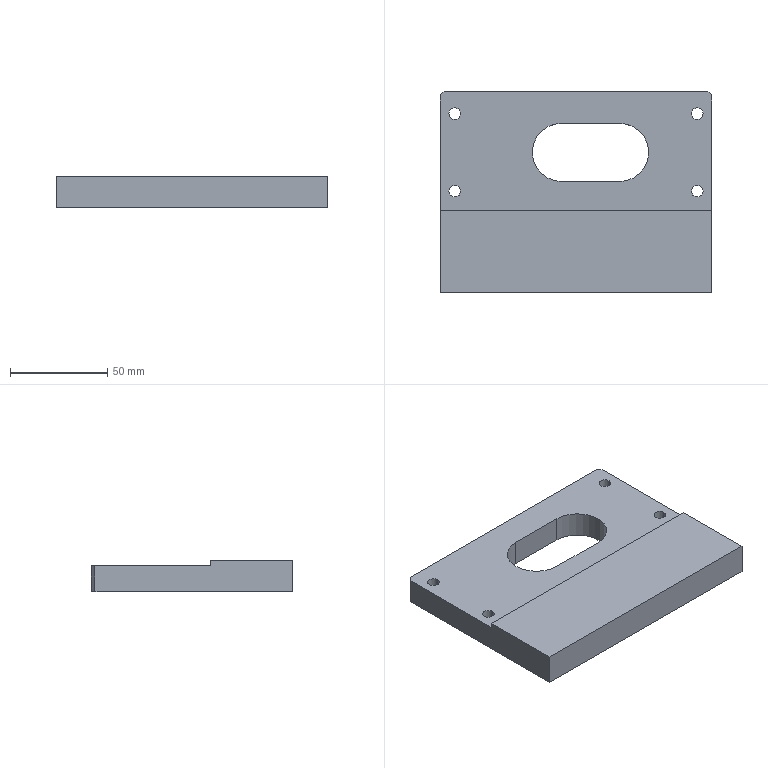Part | STEP file | [01]-2 | 1 solid | 22 faces | box 140 x 104 x 16 mm | volume 187092 mm3 | plane 12 | cylinder 10 | commonest cylinder face diameters 6 x8 30 x2
STEP:
#1=CARTESIAN_POINT('',(135.5,92.4,13.35));
#2=VERTEX_POINT('',#1);
#3=CARTESIAN_POINT('',(129.5,92.4,13.35));
#4=VERTEX_POINT('',#3);
#5=CARTESIAN_POINT('',(132.5,92.4,13.35));
#6=DIRECTION('',(0.,0.,-1.));
#7=DIRECTION('',(-1.,0.,0.));
#8=AXIS2_PLACEMENT_3D('',#5,#6,#7);
#9=CIRCLE('',#8,3.);
#10=EDGE_CURVE('',#2,#4,#9,.T.);
#11=ORIENTED_EDGE('',*,*,#10,.F.);
#12=CARTESIAN_POINT('',(135.5,92.4,0.));
#13=VERTEX_POINT('',#12);
#14=CARTESIAN_POINT('',(135.5,92.4,13.35));
#15=DIRECTION('',(0.,0.,-1.));
#16=VECTOR('',#15,1000.);
#17=LINE('',#14,#16);
#18=EDGE_CURVE('',#2,#13,#17,.T.);
#19=ORIENTED_EDGE('',*,*,#18,.T.);
#20=CARTESIAN_POINT('',(129.5,92.4,0.));
#21=VERTEX_POINT('',#20);
#22=CARTESIAN_POINT('',(132.5,92.4,0.));
#23=DIRECTION('',(0.,0.,1.));
#24=DIRECTION('',(1.,0.,0.));
#25=AXIS2_PLACEMENT_3D('',#22,#23,#24);
#26=CIRCLE('',#25,3.);
#27=EDGE_CURVE('',#21,#13,#26,.T.);
#28=ORIENTED_EDGE('',*,*,#27,.F.);
#29=CARTESIAN_POINT('',(129.5,92.4,13.35));
#30=DIRECTION('',(0.,0.,-1.));
#31=VECTOR('',#30,1000.);
#32=LINE('',#29,#31);
#33=EDGE_CURVE('',#4,#21,#32,.T.);
#34=ORIENTED_EDGE('',*,*,#33,.F.);
#35=EDGE_LOOP('',(#11,#19,#28,#34));
#36=FACE_OUTER_BOUND('',#35,.T.);
#37=CARTESIAN_POINT('',(132.5,92.4,13.35));
#38=DIRECTION('',(0.,0.,-1.));
#39=DIRECTION('',(-1.,0.,0.));
#40=AXIS2_PLACEMENT_3D('',#37,#38,#39);
#41=CYLINDRICAL_SURFACE('',#40,3.);
#42=ADVANCED_FACE('',(#36),#41,.F.);
#43=CARTESIAN_POINT('',(135.5,52.4,13.35));
#44=VERTEX_POINT('',#43);
#45=CARTESIAN_POINT('',(129.5,52.4,13.35));
#46=VERTEX_POINT('',#45);
#47=CARTESIAN_POINT('',(132.5,52.4,13.35));
#48=DIRECTION('',(0.,0.,-1.));
#49=DIRECTION('',(-1.,0.,0.));
#50=AXIS2_PLACEMENT_3D('',#47,#48,#49);
#51=CIRCLE('',#50,3.);
#52=EDGE_CURVE('',#44,#46,#51,.T.);
#53=ORIENTED_EDGE('',*,*,#52,.F.);
#54=CARTESIAN_POINT('',(135.5,52.4,0.));
#55=VERTEX_POINT('',#54);
#56=CARTESIAN_POINT('',(135.5,52.4,13.35));
#57=DIRECTION('',(0.,0.,-1.));
#58=VECTOR('',#57,1000.);
#59=LINE('',#56,#58);
#60=EDGE_CURVE('',#44,#55,#59,.T.);
#61=ORIENTED_EDGE('',*,*,#60,.T.);
#62=CARTESIAN_POINT('',(129.5,52.4,0.));
#63=VERTEX_POINT('',#62);
#64=CARTESIAN_POINT('',(132.5,52.4,0.));
#65=DIRECTION('',(0.,0.,1.));
#66=DIRECTION('',(1.,0.,0.));
#67=AXIS2_PLACEMENT_3D('',#64,#65,#66);
#68=CIRCLE('',#67,3.);
#69=EDGE_CURVE('',#63,#55,#68,.T.);
#70=ORIENTED_EDGE('',*,*,#69,.F.);
#71=CARTESIAN_POINT('',(129.5,52.4,13.35));
#72=DIRECTION('',(0.,0.,-1.));
#73=VECTOR('',#72,1000.);
#74=LINE('',#71,#73);
#75=EDGE_CURVE('',#46,#63,#74,.T.);
#76=ORIENTED_EDGE('',*,*,#75,.F.);
#77=EDGE_LOOP('',(#53,#61,#70,#76));
#78=FACE_OUTER_BOUND('',#77,.T.);
#79=CARTESIAN_POINT('',(132.5,52.4,13.35));
#80=DIRECTION('',(0.,0.,-1.));
#81=DIRECTION('',(-1.,0.,0.));
#82=AXIS2_PLACEMENT_3D('',#79,#80,#81);
#83=CYLINDRICAL_SURFACE('',#82,3.);
#84=ADVANCED_FACE('',(#78),#83,.F.);
#85=CARTESIAN_POINT('',(10.5,52.4,13.35));
#86=VERTEX_POINT('',#85);
#87=CARTESIAN_POINT('',(4.5,52.4,13.35));
#88=VERTEX_POINT('',#87);
#89=CARTESIAN_POINT('',(7.5,52.4,13.35));
#90=DIRECTION('',(0.,0.,-1.));
#91=DIRECTION('',(-1.,0.,0.));
#92=AXIS2_PLACEMENT_3D('',#89,#90,#91);
#93=CIRCLE('',#92,3.);
#94=EDGE_CURVE('',#86,#88,#93,.T.);
#95=ORIENTED_EDGE('',*,*,#94,.F.);
#96=CARTESIAN_POINT('',(10.5,52.4,0.));
#97=VERTEX_POINT('',#96);
#98=CARTESIAN_POINT('',(10.5,52.4,13.35));
#99=DIRECTION('',(0.,0.,-1.));
#100=VECTOR('',#99,1000.);
#101=LINE('',#98,#100);
#102=EDGE_CURVE('',#86,#97,#101,.T.);
#103=ORIENTED_EDGE('',*,*,#102,.T.);
#104=CARTESIAN_POINT('',(4.5,52.4,0.));
#105=VERTEX_POINT('',#104);
#106=CARTESIAN_POINT('',(7.5,52.4,0.));
#107=DIRECTION('',(0.,0.,1.));
#108=DIRECTION('',(1.,0.,0.));
#109=AXIS2_PLACEMENT_3D('',#106,#107,#108);
#110=CIRCLE('',#109,3.);
#111=EDGE_CURVE('',#105,#97,#110,.T.);
#112=ORIENTED_EDGE('',*,*,#111,.F.);
#113=CARTESIAN_POINT('',(4.5,52.4,13.35));
#114=DIRECTION('',(0.,0.,-1.));
#115=VECTOR('',#114,1000.);
#116=LINE('',#113,#115);
#117=EDGE_CURVE('',#88,#105,#116,.T.);
#118=ORIENTED_EDGE('',*,*,#117,.F.);
#119=EDGE_LOOP('',(#95,#103,#112,#118));
#120=FACE_OUTER_BOUND('',#119,.T.);
#121=CARTESIAN_POINT('',(7.5,52.4,13.35));
#122=DIRECTION('',(0.,0.,-1.));
#123=DIRECTION('',(-1.,0.,0.));
#124=AXIS2_PLACEMENT_3D('',#121,#122,#123);
#125=CYLINDRICAL_SURFACE('',#124,3.);
#126=ADVANCED_FACE('',(#120),#125,.F.);
#127=CARTESIAN_POINT('',(10.5,92.4,13.35));
#128=VERTEX_POINT('',#127);
#129=CARTESIAN_POINT('',(4.5,92.4,13.35));
#130=VERTEX_POINT('',#129);
#131=CARTESIAN_POINT('',(7.5,92.4,13.35));
#132=DIRECTION('',(0.,0.,-1.));
#133=DIRECTION('',(-1.,0.,0.));
#134=AXIS2_PLACEMENT_3D('',#131,#132,#133);
#135=CIRCLE('',#134,3.);
#136=EDGE_CURVE('',#128,#130,#135,.T.);
#137=ORIENTED_EDGE('',*,*,#136,.F.);
#138=CARTESIAN_POINT('',(10.5,92.4,0.));
#139=VERTEX_POINT('',#138);
#140=CARTESIAN_POINT('',(10.5,92.4,13.35));
#141=DIRECTION('',(0.,0.,-1.));
#142=VECTOR('',#141,1000.);
#143=LINE('',#140,#142);
#144=EDGE_CURVE('',#128,#139,#143,.T.);
#145=ORIENTED_EDGE('',*,*,#144,.T.);
#146=CARTESIAN_POINT('',(4.5,92.4,0.));
#147=VERTEX_POINT('',#146);
#148=CARTESIAN_POINT('',(7.5,92.4,0.));
#149=DIRECTION('',(0.,0.,1.));
#150=DIRECTION('',(1.,0.,0.));
#151=AXIS2_PLACEMENT_3D('',#148,#149,#150);
#152=CIRCLE('',#151,3.);
#153=EDGE_CURVE('',#147,#139,#152,.T.);
#154=ORIENTED_EDGE('',*,*,#153,.F.);
#155=CARTESIAN_POINT('',(4.5,92.4,13.35));
#156=DIRECTION('',(0.,0.,-1.));
#157=VECTOR('',#156,1000.);
#158=LINE('',#155,#157);
#159=EDGE_CURVE('',#130,#147,#158,.T.);
#160=ORIENTED_EDGE('',*,*,#159,.F.);
#161=EDGE_LOOP('',(#137,#145,#154,#160));
#162=FACE_OUTER_BOUND('',#161,.T.);
#163=CARTESIAN_POINT('',(7.5,92.4,13.35));
#164=DIRECTION('',(0.,0.,-1.));
#165=DIRECTION('',(-1.,0.,0.));
#166=AXIS2_PLACEMENT_3D('',#163,#164,#165);
#167=CYLINDRICAL_SURFACE('',#166,3.);
#168=ADVANCED_FACE('',(#162),#167,.F.);
#169=CARTESIAN_POINT('',(138.,104.,13.35));
#170=VERTEX_POINT('',#169);
#171=CARTESIAN_POINT('',(2.,104.,13.35));
#172=VERTEX_POINT('',#171);
#173=CARTESIAN_POINT('',(0.,104.,13.35));
#174=DIRECTION('',(-1.,0.,0.));
#175=VECTOR('',#174,1000.);
#176=LINE('',#173,#175);
#177=EDGE_CURVE('',#170,#172,#176,.T.);
#178=ORIENTED_EDGE('',*,*,#177,.F.);
#179=CARTESIAN_POINT('',(138.,104.,0.));
#180=VERTEX_POINT('',#179);
#181=CARTESIAN_POINT('',(138.,104.,0.));
#182=DIRECTION('',(0.,0.,-1.));
#183=VECTOR('',#182,1000.);
#184=LINE('',#181,#183);
#185=EDGE_CURVE('',#170,#180,#184,.T.);
#186=ORIENTED_EDGE('',*,*,#185,.T.);
#187=CARTESIAN_POINT('',(2.,104.,0.));
#188=VERTEX_POINT('',#187);
#189=CARTESIAN_POINT('',(0.,104.,0.));
#190=DIRECTION('',(1.,0.,0.));
#191=VECTOR('',#190,1000.);
#192=LINE('',#189,#191);
#193=EDGE_CURVE('',#188,#180,#192,.T.);
#194=ORIENTED_EDGE('',*,*,#193,.F.);
#195=CARTESIAN_POINT('',(2.,104.,16.));
#196=DIRECTION('',(0.,0.,1.));
#197=VECTOR('',#196,1000.);
#198=LINE('',#195,#197);
#199=EDGE_CURVE('',#188,#172,#198,.T.);
#200=ORIENTED_EDGE('',*,*,#199,.T.);
#201=EDGE_LOOP('',(#178,#186,#194,#200));
#202=FACE_OUTER_BOUND('',#201,.T.);
#203=CARTESIAN_POINT('',(0.,104.,0.));
#204=DIRECTION('',(0.,1.,0.));
#205=DIRECTION('',(-1.,0.,0.));
#206=AXIS2_PLACEMENT_3D('',#203,#204,#205);
#207=PLANE('',#206);
#208=ADVANCED_FACE('',(#202),#207,.T.);
#209=CARTESIAN_POINT('',(0.,42.4,16.));
#210=VERTEX_POINT('',#209);
#211=CARTESIAN_POINT('',(140.,42.4,16.));
#212=VERTEX_POINT('',#211);
#213=CARTESIAN_POINT('',(0.,42.4,16.));
#214=DIRECTION('',(1.,0.,0.));
#215=VECTOR('',#214,1000.);
#216=LINE('',#213,#215);
#217=EDGE_CURVE('',#210,#212,#216,.T.);
#218=ORIENTED_EDGE('',*,*,#217,.F.);
#219=CARTESIAN_POINT('',(0.,0.,16.));
#220=VERTEX_POINT('',#219);
#221=CARTESIAN_POINT('',(0.,104.,16.));
#222=DIRECTION('',(0.,-1.,0.));
#223=VECTOR('',#222,1000.);
#224=LINE('',#221,#223);
#225=EDGE_CURVE('',#210,#220,#224,.T.);
#226=ORIENTED_EDGE('',*,*,#225,.T.);
#227=CARTESIAN_POINT('',(140.,0.,16.));
#228=VERTEX_POINT('',#227);
#229=CARTESIAN_POINT('',(0.,0.,16.));
#230=DIRECTION('',(1.,0.,0.));
#231=VECTOR('',#230,1000.);
#232=LINE('',#229,#231);
#233=EDGE_CURVE('',#220,#228,#232,.T.);
#234=ORIENTED_EDGE('',*,*,#233,.T.);
#235=CARTESIAN_POINT('',(140.,104.,16.));
#236=DIRECTION('',(0.,-1.,0.));
#237=VECTOR('',#236,1000.);
#238=LINE('',#235,#237);
#239=EDGE_CURVE('',#212,#228,#238,.T.);
#240=ORIENTED_EDGE('',*,*,#239,.F.);
#241=EDGE_LOOP('',(#218,#226,#234,#240));
#242=FACE_OUTER_BOUND('',#241,.T.);
#243=CARTESIAN_POINT('',(0.,104.,16.));
#244=DIRECTION('',(0.,0.,1.));
#245=DIRECTION('',(0.,-1.,0.));
#246=AXIS2_PLACEMENT_3D('',#243,#244,#245);
#247=PLANE('',#246);
#248=ADVANCED_FACE('',(#242),#247,.T.);
#249=CARTESIAN_POINT('',(140.,0.,0.));
#250=VERTEX_POINT('',#249);
#251=CARTESIAN_POINT('',(140.,0.,16.));
#252=DIRECTION('',(0.,0.,-1.));
#253=VECTOR('',#252,1000.);
#254=LINE('',#251,#253);
#255=EDGE_CURVE('',#228,#250,#254,.T.);
#256=ORIENTED_EDGE('',*,*,#255,.F.);
#257=ORIENTED_EDGE('',*,*,#233,.F.);
#258=CARTESIAN_POINT('',(0.,0.,0.));
#259=VERTEX_POINT('',#258);
#260=CARTESIAN_POINT('',(0.,0.,16.));
#261=DIRECTION('',(0.,0.,-1.));
#262=VECTOR('',#261,1000.);
#263=LINE('',#260,#262);
#264=EDGE_CURVE('',#220,#259,#263,.T.);
#265=ORIENTED_EDGE('',*,*,#264,.T.);
#266=CARTESIAN_POINT('',(0.,0.,0.));
#267=DIRECTION('',(1.,0.,0.));
#268=VECTOR('',#267,1000.);
#269=LINE('',#266,#268);
#270=EDGE_CURVE('',#259,#250,#269,.T.);
#271=ORIENTED_EDGE('',*,*,#270,.T.);
#272=EDGE_LOOP('',(#256,#257,#265,#271));
#273=FACE_OUTER_BOUND('',#272,.T.);
#274=CARTESIAN_POINT('',(0.,0.,16.));
#275=DIRECTION('',(0.,-1.,0.));
#276=DIRECTION('',(1.,0.,0.));
#277=AXIS2_PLACEMENT_3D('',#274,#275,#276);
#278=PLANE('',#277);
#279=ADVANCED_FACE('',(#273),#278,.T.);
#280=ORIENTED_EDGE('',*,*,#27,.T.);
#281=CARTESIAN_POINT('',(132.5,92.4,0.));
#282=DIRECTION('',(0.,0.,1.));
#283=DIRECTION('',(1.,0.,0.));
#284=AXIS2_PLACEMENT_3D('',#281,#282,#283);
#285=CIRCLE('',#284,3.);
#286=EDGE_CURVE('',#13,#21,#285,.T.);
#287=ORIENTED_EDGE('',*,*,#286,.T.);
#288=EDGE_LOOP('',(#280,#287));
#289=FACE_BOUND('',#288,.T.);
#290=ORIENTED_EDGE('',*,*,#69,.T.);
#291=CARTESIAN_POINT('',(132.5,52.4,0.));
#292=DIRECTION('',(0.,0.,1.));
#293=DIRECTION('',(1.,0.,0.));
#294=AXIS2_PLACEMENT_3D('',#291,#292,#293);
#295=CIRCLE('',#294,3.);
#296=EDGE_CURVE('',#55,#63,#295,.T.);
#297=ORIENTED_EDGE('',*,*,#296,.T.);
#298=EDGE_LOOP('',(#290,#297));
#299=FACE_BOUND('',#298,.T.);
#300=ORIENTED_EDGE('',*,*,#111,.T.);
#301=CARTESIAN_POINT('',(7.5,52.4,0.));
#302=DIRECTION('',(0.,0.,1.));
#303=DIRECTION('',(1.,0.,0.));
#304=AXIS2_PLACEMENT_3D('',#301,#302,#303);
#305=CIRCLE('',#304,3.);
#306=EDGE_CURVE('',#97,#105,#305,.T.);
#307=ORIENTED_EDGE('',*,*,#306,.T.);
#308=EDGE_LOOP('',(#300,#307));
#309=FACE_BOUND('',#308,.T.);
#310=ORIENTED_EDGE('',*,*,#153,.T.);
#311=CARTESIAN_POINT('',(7.5,92.4,0.));
#312=DIRECTION('',(0.,0.,1.));
#313=DIRECTION('',(1.,0.,0.));
#314=AXIS2_PLACEMENT_3D('',#311,#312,#313);
#315=CIRCLE('',#314,3.);
#316=EDGE_CURVE('',#139,#147,#315,.T.);
#317=ORIENTED_EDGE('',*,*,#316,.T.);
#318=EDGE_LOOP('',(#310,#317));
#319=FACE_BOUND('',#318,.T.);
#320=CARTESIAN_POINT('',(62.5,87.4,0.));
#321=VERTEX_POINT('',#320);
#322=CARTESIAN_POINT('',(62.5,57.4,0.));
#323=VERTEX_POINT('',#322);
#324=CARTESIAN_POINT('',(62.5,72.4,0.));
#325=DIRECTION('',(0.,0.,1.));
#326=DIRECTION('',(0.,1.,0.));
#327=AXIS2_PLACEMENT_3D('',#324,#325,#326);
#328=CIRCLE('',#327,15.);
#329=EDGE_CURVE('',#321,#323,#328,.T.);
#330=ORIENTED_EDGE('',*,*,#329,.T.);
#331=CARTESIAN_POINT('',(92.5,57.4,0.));
#332=VERTEX_POINT('',#331);
#333=CARTESIAN_POINT('',(0.,57.4,0.));
#334=DIRECTION('',(-1.,0.,0.));
#335=VECTOR('',#334,1000.);
#336=LINE('',#333,#335);
#337=EDGE_CURVE('',#332,#323,#336,.T.);
#338=ORIENTED_EDGE('',*,*,#337,.F.);
#339=CARTESIAN_POINT('',(92.5,87.4,0.));
#340=VERTEX_POINT('',#339);
#341=CARTESIAN_POINT('',(92.5,72.4,0.));
#342=DIRECTION('',(0.,0.,1.));
#343=DIRECTION('',(0.,1.,0.));
#344=AXIS2_PLACEMENT_3D('',#341,#342,#343);
#345=CIRCLE('',#344,15.);
#346=EDGE_CURVE('',#332,#340,#345,.T.);
#347=ORIENTED_EDGE('',*,*,#346,.T.);
#348=CARTESIAN_POINT('',(0.,87.4,0.));
#349=DIRECTION('',(1.,0.,0.));
#350=VECTOR('',#349,1000.);
#351=LINE('',#348,#350);
#352=EDGE_CURVE('',#321,#340,#351,.T.);
#353=ORIENTED_EDGE('',*,*,#352,.F.);
#354=EDGE_LOOP('',(#330,#338,#347,#353));
#355=FACE_BOUND('',#354,.T.);
#356=CARTESIAN_POINT('',(0.,102.,0.));
#357=VERTEX_POINT('',#356);
#358=CARTESIAN_POINT('',(0.,0.,0.));
#359=DIRECTION('',(0.,1.,0.));
#360=VECTOR('',#359,1000.);
#361=LINE('',#358,#360);
#362=EDGE_CURVE('',#259,#357,#361,.T.);
#363=ORIENTED_EDGE('',*,*,#362,.T.);
#364=CARTESIAN_POINT('',(-51.,51.,0.));
#365=DIRECTION('',(0.7071,0.7071,0.));
#366=VECTOR('',#365,1000.);
#367=LINE('',#364,#366);
#368=EDGE_CURVE('',#357,#188,#367,.T.);
#369=ORIENTED_EDGE('',*,*,#368,.T.);
#370=ORIENTED_EDGE('',*,*,#193,.T.);
#371=CARTESIAN_POINT('',(140.,102.,0.));
#372=VERTEX_POINT('',#371);
#373=CARTESIAN_POINT('',(121.,121.,0.));
#374=DIRECTION('',(0.7071,-0.7071,0.));
#375=VECTOR('',#374,1000.);
#376=LINE('',#373,#375);
#377=EDGE_CURVE('',#180,#372,#376,.T.);
#378=ORIENTED_EDGE('',*,*,#377,.T.);
#379=CARTESIAN_POINT('',(140.,0.,0.));
#380=DIRECTION('',(0.,1.,0.));
#381=VECTOR('',#380,1000.);
#382=LINE('',#379,#381);
#383=EDGE_CURVE('',#250,#372,#382,.T.);
#384=ORIENTED_EDGE('',*,*,#383,.F.);
#385=ORIENTED_EDGE('',*,*,#270,.F.);
#386=EDGE_LOOP('',(#363,#369,#370,#378,#384,#385));
#387=FACE_OUTER_BOUND('',#386,.T.);
#388=CARTESIAN_POINT('',(0.,0.,0.));
#389=DIRECTION('',(0.,0.,-1.));
#390=DIRECTION('',(0.,1.,0.));
#391=AXIS2_PLACEMENT_3D('',#388,#389,#390);
#392=PLANE('',#391);
#393=ADVANCED_FACE('',(#289,#299,#309,#319,#355,#387),#392,.T.);
#394=ORIENTED_EDGE('',*,*,#225,.F.);
#395=CARTESIAN_POINT('',(0.,42.4,13.35));
#396=VERTEX_POINT('',#395);
#397=CARTESIAN_POINT('',(0.,42.4,-87.886));
#398=DIRECTION('',(0.,0.,-1.));
#399=VECTOR('',#398,1000.);
#400=LINE('',#397,#399);
#401=EDGE_CURVE('',#210,#396,#400,.T.);
#402=ORIENTED_EDGE('',*,*,#401,.T.);
#403=CARTESIAN_POINT('',(0.,102.,13.35));
#404=VERTEX_POINT('',#403);
#405=CARTESIAN_POINT('',(0.,329.827,13.35));
#406=DIRECTION('',(0.,1.,0.));
#407=VECTOR('',#406,1000.);
#408=LINE('',#405,#407);
#409=EDGE_CURVE('',#396,#404,#408,.T.);
#410=ORIENTED_EDGE('',*,*,#409,.T.);
#411=CARTESIAN_POINT('',(0.,102.,0.));
#412=DIRECTION('',(0.,0.,-1.));
#413=VECTOR('',#412,1000.);
#414=LINE('',#411,#413);
#415=EDGE_CURVE('',#404,#357,#414,.T.);
#416=ORIENTED_EDGE('',*,*,#415,.T.);
#417=ORIENTED_EDGE('',*,*,#362,.F.);
#418=ORIENTED_EDGE('',*,*,#264,.F.);
#419=EDGE_LOOP('',(#394,#402,#410,#416,#417,#418));
#420=FACE_OUTER_BOUND('',#419,.T.);
#421=CARTESIAN_POINT('',(0.,329.827,-87.886));
#422=DIRECTION('',(1.,0.,0.));
#423=DIRECTION('',(0.,1.,0.));
#424=AXIS2_PLACEMENT_3D('',#421,#422,#423);
#425=PLANE('',#424);
#426=ADVANCED_FACE('',(#420),#425,.F.);
#427=CARTESIAN_POINT('',(140.,42.4,13.35));
#428=VERTEX_POINT('',#427);
#429=CARTESIAN_POINT('',(140.,102.,13.35));
#430=VERTEX_POINT('',#429);
#431=CARTESIAN_POINT('',(140.,81.4,13.35));
#432=DIRECTION('',(0.,1.,0.));
#433=VECTOR('',#432,1000.);
#434=LINE('',#431,#433);
#435=EDGE_CURVE('',#428,#430,#434,.T.);
#436=ORIENTED_EDGE('',*,*,#435,.F.);
#437=CARTESIAN_POINT('',(140.,42.4,13.35));
#438=DIRECTION('',(0.,0.,1.));
#439=VECTOR('',#438,1000.);
#440=LINE('',#437,#439);
#441=EDGE_CURVE('',#428,#212,#440,.T.);
#442=ORIENTED_EDGE('',*,*,#441,.T.);
#443=ORIENTED_EDGE('',*,*,#239,.T.);
#444=ORIENTED_EDGE('',*,*,#255,.T.);
#445=ORIENTED_EDGE('',*,*,#383,.T.);
#446=CARTESIAN_POINT('',(140.,102.,-87.886));
#447=DIRECTION('',(0.,0.,1.));
#448=VECTOR('',#447,1000.);
#449=LINE('',#446,#448);
#450=EDGE_CURVE('',#372,#430,#449,.T.);
#451=ORIENTED_EDGE('',*,*,#450,.T.);
#452=EDGE_LOOP('',(#436,#442,#443,#444,#445,#451));
#453=FACE_OUTER_BOUND('',#452,.T.);
#454=CARTESIAN_POINT('',(140.,329.827,-87.886));
#455=DIRECTION('',(1.,0.,0.));
#456=DIRECTION('',(0.,1.,0.));
#457=AXIS2_PLACEMENT_3D('',#454,#455,#456);
#458=PLANE('',#457);
#459=ADVANCED_FACE('',(#453),#458,.T.);
#460=CARTESIAN_POINT('',(140.,102.,13.35));
#461=DIRECTION('',(-0.7071,0.7071,0.));
#462=VECTOR('',#461,1000.);
#463=LINE('',#460,#462);
#464=EDGE_CURVE('',#430,#170,#463,.T.);
#465=ORIENTED_EDGE('',*,*,#464,.F.);
#466=ORIENTED_EDGE('',*,*,#450,.F.);
#467=ORIENTED_EDGE('',*,*,#377,.F.);
#468=ORIENTED_EDGE('',*,*,#185,.F.);
#469=EDGE_LOOP('',(#465,#466,#467,#468));
#470=FACE_OUTER_BOUND('',#469,.T.);
#471=CARTESIAN_POINT('',(140.,102.,-87.886));
#472=DIRECTION('',(-0.7071,-0.7071,0.));
#473=DIRECTION('',(0.,0.,1.));
#474=AXIS2_PLACEMENT_3D('',#471,#472,#473);
#475=PLANE('',#474);
#476=ADVANCED_FACE('',(#470),#475,.F.);
#477=CARTESIAN_POINT('',(2.,104.,13.35));
#478=DIRECTION('',(-0.7071,-0.7071,0.));
#479=VECTOR('',#478,1000.);
#480=LINE('',#477,#479);
#481=EDGE_CURVE('',#172,#404,#480,.T.);
#482=ORIENTED_EDGE('',*,*,#481,.F.);
#483=ORIENTED_EDGE('',*,*,#199,.F.);
#484=ORIENTED_EDGE('',*,*,#368,.F.);
#485=ORIENTED_EDGE('',*,*,#415,.F.);
#486=EDGE_LOOP('',(#482,#483,#484,#485));
#487=FACE_OUTER_BOUND('',#486,.T.);
#488=CARTESIAN_POINT('',(2.,104.,0.));
#489=DIRECTION('',(-0.7071,0.7071,0.));
#490=DIRECTION('',(0.,0.,-1.));
#491=AXIS2_PLACEMENT_3D('',#488,#489,#490);
#492=PLANE('',#491);
#493=ADVANCED_FACE('',(#487),#492,.T.);
#494=CARTESIAN_POINT('',(132.5,92.4,13.35));
#495=DIRECTION('',(0.,0.,-1.));
#496=DIRECTION('',(-1.,0.,0.));
#497=AXIS2_PLACEMENT_3D('',#494,#495,#496);
#498=CIRCLE('',#497,3.);
#499=EDGE_CURVE('',#4,#2,#498,.T.);
#500=ORIENTED_EDGE('',*,*,#499,.T.);
#501=ORIENTED_EDGE('',*,*,#10,.T.);
#502=EDGE_LOOP('',(#500,#501));
#503=FACE_BOUND('',#502,.T.);
#504=CARTESIAN_POINT('',(132.5,52.4,13.35));
#505=DIRECTION('',(0.,0.,-1.));
#506=DIRECTION('',(-1.,0.,0.));
#507=AXIS2_PLACEMENT_3D('',#504,#505,#506);
#508=CIRCLE('',#507,3.);
#509=EDGE_CURVE('',#46,#44,#508,.T.);
#510=ORIENTED_EDGE('',*,*,#509,.T.);
#511=ORIENTED_EDGE('',*,*,#52,.T.);
#512=EDGE_LOOP('',(#510,#511));
#513=FACE_BOUND('',#512,.T.);
#514=CARTESIAN_POINT('',(7.5,52.4,13.35));
#515=DIRECTION('',(0.,0.,-1.));
#516=DIRECTION('',(-1.,0.,0.));
#517=AXIS2_PLACEMENT_3D('',#514,#515,#516);
#518=CIRCLE('',#517,3.);
#519=EDGE_CURVE('',#88,#86,#518,.T.);
#520=ORIENTED_EDGE('',*,*,#519,.T.);
#521=ORIENTED_EDGE('',*,*,#94,.T.);
#522=EDGE_LOOP('',(#520,#521));
#523=FACE_BOUND('',#522,.T.);
#524=CARTESIAN_POINT('',(7.5,92.4,13.35));
#525=DIRECTION('',(0.,0.,-1.));
#526=DIRECTION('',(-1.,0.,0.));
#527=AXIS2_PLACEMENT_3D('',#524,#525,#526);
#528=CIRCLE('',#527,3.);
#529=EDGE_CURVE('',#130,#128,#528,.T.);
#530=ORIENTED_EDGE('',*,*,#529,.T.);
#531=ORIENTED_EDGE('',*,*,#136,.T.);
#532=EDGE_LOOP('',(#530,#531));
#533=FACE_BOUND('',#532,.T.);
#534=ORIENTED_EDGE('',*,*,#464,.T.);
#535=ORIENTED_EDGE('',*,*,#177,.T.);
#536=ORIENTED_EDGE('',*,*,#481,.T.);
#537=ORIENTED_EDGE('',*,*,#409,.F.);
#538=CARTESIAN_POINT('',(55.,42.4,13.35));
#539=DIRECTION('',(1.,0.,0.));
#540=VECTOR('',#539,1000.);
#541=LINE('',#538,#540);
#542=EDGE_CURVE('',#396,#428,#541,.T.);
#543=ORIENTED_EDGE('',*,*,#542,.T.);
#544=ORIENTED_EDGE('',*,*,#435,.T.);
#545=EDGE_LOOP('',(#534,#535,#536,#537,#543,#544));
#546=FACE_OUTER_BOUND('',#545,.T.);
#547=CARTESIAN_POINT('',(92.5,57.4,13.35));
#548=VERTEX_POINT('',#547);
#549=CARTESIAN_POINT('',(62.5,57.4,13.35));
#550=VERTEX_POINT('',#549);
#551=CARTESIAN_POINT('',(77.5,57.4,13.35));
#552=DIRECTION('',(-1.,0.,0.));
#553=VECTOR('',#552,1000.);
#554=LINE('',#551,#553);
#555=EDGE_CURVE('',#548,#550,#554,.T.);
#556=ORIENTED_EDGE('',*,*,#555,.T.);
#557=CARTESIAN_POINT('',(62.5,87.4,13.35));
#558=VERTEX_POINT('',#557);
#559=CARTESIAN_POINT('',(62.5,72.4,13.35));
#560=DIRECTION('',(0.,0.,-1.));
#561=DIRECTION('',(0.,1.,0.));
#562=AXIS2_PLACEMENT_3D('',#559,#560,#561);
#563=CIRCLE('',#562,15.);
#564=EDGE_CURVE('',#550,#558,#563,.T.);
#565=ORIENTED_EDGE('',*,*,#564,.T.);
#566=CARTESIAN_POINT('',(92.5,87.4,13.35));
#567=VERTEX_POINT('',#566);
#568=CARTESIAN_POINT('',(77.5,87.4,13.35));
#569=DIRECTION('',(1.,0.,0.));
#570=VECTOR('',#569,1000.);
#571=LINE('',#568,#570);
#572=EDGE_CURVE('',#558,#567,#571,.T.);
#573=ORIENTED_EDGE('',*,*,#572,.T.);
#574=CARTESIAN_POINT('',(92.5,72.4,13.35));
#575=DIRECTION('',(0.,0.,-1.));
#576=DIRECTION('',(0.,1.,0.));
#577=AXIS2_PLACEMENT_3D('',#574,#575,#576);
#578=CIRCLE('',#577,15.);
#579=EDGE_CURVE('',#567,#548,#578,.T.);
#580=ORIENTED_EDGE('',*,*,#579,.T.);
#581=EDGE_LOOP('',(#556,#565,#573,#580));
#582=FACE_BOUND('',#581,.T.);
#583=CARTESIAN_POINT('',(55.,81.4,13.35));
#584=DIRECTION('',(0.,0.,-1.));
#585=DIRECTION('',(-1.,0.,0.));
#586=AXIS2_PLACEMENT_3D('',#583,#584,#585);
#587=PLANE('',#586);
#588=ADVANCED_FACE('',(#503,#513,#523,#533,#546,#582),#587,.F.);
#589=ORIENTED_EDGE('',*,*,#217,.T.);
#590=ORIENTED_EDGE('',*,*,#441,.F.);
#591=ORIENTED_EDGE('',*,*,#542,.F.);
#592=ORIENTED_EDGE('',*,*,#401,.F.);
#593=EDGE_LOOP('',(#589,#590,#591,#592));
#594=FACE_OUTER_BOUND('',#593,.T.);
#595=CARTESIAN_POINT('',(55.,42.4,13.35));
#596=DIRECTION('',(0.,-1.,0.));
#597=DIRECTION('',(0.,0.,-1.));
#598=AXIS2_PLACEMENT_3D('',#595,#596,#597);
#599=PLANE('',#598);
#600=ADVANCED_FACE('',(#594),#599,.F.);
#601=ORIENTED_EDGE('',*,*,#572,.F.);
#602=CARTESIAN_POINT('',(62.5,87.4,0.));
#603=DIRECTION('',(0.,0.,-1.));
#604=VECTOR('',#603,1000.);
#605=LINE('',#602,#604);
#606=EDGE_CURVE('',#558,#321,#605,.T.);
#607=ORIENTED_EDGE('',*,*,#606,.T.);
#608=ORIENTED_EDGE('',*,*,#352,.T.);
#609=CARTESIAN_POINT('',(92.5,87.4,13.35));
#610=DIRECTION('',(0.,0.,1.));
#611=VECTOR('',#610,1000.);
#612=LINE('',#609,#611);
#613=EDGE_CURVE('',#340,#567,#612,.T.);
#614=ORIENTED_EDGE('',*,*,#613,.T.);
#615=EDGE_LOOP('',(#601,#607,#608,#614));
#616=FACE_OUTER_BOUND('',#615,.T.);
#617=CARTESIAN_POINT('',(77.5,87.4,-6.65));
#618=DIRECTION('',(0.,1.,0.));
#619=DIRECTION('',(0.,0.,-1.));
#620=AXIS2_PLACEMENT_3D('',#617,#618,#619);
#621=PLANE('',#620);
#622=ADVANCED_FACE('',(#616),#621,.F.);
#623=ORIENTED_EDGE('',*,*,#337,.T.);
#624=CARTESIAN_POINT('',(62.5,57.4,13.35));
#625=DIRECTION('',(0.,0.,1.));
#626=VECTOR('',#625,1000.);
#627=LINE('',#624,#626);
#628=EDGE_CURVE('',#323,#550,#627,.T.);
#629=ORIENTED_EDGE('',*,*,#628,.T.);
#630=ORIENTED_EDGE('',*,*,#555,.F.);
#631=CARTESIAN_POINT('',(92.5,57.4,0.));
#632=DIRECTION('',(0.,0.,-1.));
#633=VECTOR('',#632,1000.);
#634=LINE('',#631,#633);
#635=EDGE_CURVE('',#548,#332,#634,.T.);
#636=ORIENTED_EDGE('',*,*,#635,.T.);
#637=EDGE_LOOP('',(#623,#629,#630,#636));
#638=FACE_OUTER_BOUND('',#637,.T.);
#639=CARTESIAN_POINT('',(77.5,57.4,-6.65));
#640=DIRECTION('',(0.,-1.,0.));
#641=DIRECTION('',(0.,0.,1.));
#642=AXIS2_PLACEMENT_3D('',#639,#640,#641);
#643=PLANE('',#642);
#644=ADVANCED_FACE('',(#638),#643,.F.);
#645=ORIENTED_EDGE('',*,*,#628,.F.);
#646=ORIENTED_EDGE('',*,*,#329,.F.);
#647=ORIENTED_EDGE('',*,*,#606,.F.);
#648=ORIENTED_EDGE('',*,*,#564,.F.);
#649=EDGE_LOOP('',(#645,#646,#647,#648));
#650=FACE_OUTER_BOUND('',#649,.T.);
#651=CARTESIAN_POINT('',(62.5,72.4,-6.65));
#652=DIRECTION('',(0.,0.,-1.));
#653=DIRECTION('',(0.,1.,0.));
#654=AXIS2_PLACEMENT_3D('',#651,#652,#653);
#655=CYLINDRICAL_SURFACE('',#654,15.);
#656=ADVANCED_FACE('',(#650),#655,.F.);
#657=ORIENTED_EDGE('',*,*,#635,.F.);
#658=ORIENTED_EDGE('',*,*,#579,.F.);
#659=ORIENTED_EDGE('',*,*,#613,.F.);
#660=ORIENTED_EDGE('',*,*,#346,.F.);
#661=EDGE_LOOP('',(#657,#658,#659,#660));
#662=FACE_OUTER_BOUND('',#661,.T.);
#663=CARTESIAN_POINT('',(92.5,72.4,-6.65));
#664=DIRECTION('',(0.,0.,-1.));
#665=DIRECTION('',(0.,1.,0.));
#666=AXIS2_PLACEMENT_3D('',#663,#664,#665);
#667=CYLINDRICAL_SURFACE('',#666,15.);
#668=ADVANCED_FACE('',(#662),#667,.F.);
#669=ORIENTED_EDGE('',*,*,#144,.F.);
#670=ORIENTED_EDGE('',*,*,#529,.F.);
#671=ORIENTED_EDGE('',*,*,#159,.T.);
#672=ORIENTED_EDGE('',*,*,#316,.F.);
#673=EDGE_LOOP('',(#669,#670,#671,#672));
#674=FACE_OUTER_BOUND('',#673,.T.);
#675=CARTESIAN_POINT('',(7.5,92.4,13.35));
#676=DIRECTION('',(0.,0.,-1.));
#677=DIRECTION('',(-1.,0.,0.));
#678=AXIS2_PLACEMENT_3D('',#675,#676,#677);
#679=CYLINDRICAL_SURFACE('',#678,3.);
#680=ADVANCED_FACE('',(#674),#679,.F.);
#681=ORIENTED_EDGE('',*,*,#102,.F.);
#682=ORIENTED_EDGE('',*,*,#519,.F.);
#683=ORIENTED_EDGE('',*,*,#117,.T.);
#684=ORIENTED_EDGE('',*,*,#306,.F.);
#685=EDGE_LOOP('',(#681,#682,#683,#684));
#686=FACE_OUTER_BOUND('',#685,.T.);
#687=CARTESIAN_POINT('',(7.5,52.4,13.35));
#688=DIRECTION('',(0.,0.,-1.));
#689=DIRECTION('',(-1.,0.,0.));
#690=AXIS2_PLACEMENT_3D('',#687,#688,#689);
#691=CYLINDRICAL_SURFACE('',#690,3.);
#692=ADVANCED_FACE('',(#686),#691,.F.);
#693=ORIENTED_EDGE('',*,*,#60,.F.);
#694=ORIENTED_EDGE('',*,*,#509,.F.);
#695=ORIENTED_EDGE('',*,*,#75,.T.);
#696=ORIENTED_EDGE('',*,*,#296,.F.);
#697=EDGE_LOOP('',(#693,#694,#695,#696));
#698=FACE_OUTER_BOUND('',#697,.T.);
#699=CARTESIAN_POINT('',(132.5,52.4,13.35));
#700=DIRECTION('',(0.,0.,-1.));
#701=DIRECTION('',(-1.,0.,0.));
#702=AXIS2_PLACEMENT_3D('',#699,#700,#701);
#703=CYLINDRICAL_SURFACE('',#702,3.);
#704=ADVANCED_FACE('',(#698),#703,.F.);
#705=ORIENTED_EDGE('',*,*,#18,.F.);
#706=ORIENTED_EDGE('',*,*,#499,.F.);
#707=ORIENTED_EDGE('',*,*,#33,.T.);
#708=ORIENTED_EDGE('',*,*,#286,.F.);
#709=EDGE_LOOP('',(#705,#706,#707,#708));
#710=FACE_OUTER_BOUND('',#709,.T.);
#711=CARTESIAN_POINT('',(132.5,92.4,13.35));
#712=DIRECTION('',(0.,0.,-1.));
#713=DIRECTION('',(-1.,0.,0.));
#714=AXIS2_PLACEMENT_3D('',#711,#712,#713);
#715=CYLINDRICAL_SURFACE('',#714,3.);
#716=ADVANCED_FACE('',(#710),#715,.F.);
#717=CLOSED_SHELL('',(#42,#84,#126,#168,#208,#248,#279,#393,#426,#459,#476,#493,#588,#600,#622,#644,#656,#668,#680,#692,#704,#716));
#718=MANIFOLD_SOLID_BREP('',#717);
#719=CARTESIAN_POINT('',(0.,0.,0.));
#720=DIRECTION('',(0.,0.,1.));
#721=DIRECTION('',(1.,0.,0.));
#722=AXIS2_PLACEMENT_3D('',#719,#720,#721);
#723=(LENGTH_UNIT()NAMED_UNIT(*)SI_UNIT(.MILLI.,.METRE.));
#724=UNCERTAINTY_MEASURE_WITH_UNIT(LENGTH_MEASURE(0.00001),#723,'','');
#725=(NAMED_UNIT(*)PLANE_ANGLE_UNIT()SI_UNIT($,.RADIAN.));
#726=(NAMED_UNIT(*)SI_UNIT($,.STERADIAN.)SOLID_ANGLE_UNIT());
#727=(GEOMETRIC_REPRESENTATION_CONTEXT(3)GLOBAL_UNCERTAINTY_ASSIGNED_CONTEXT((#724))GLOBAL_UNIT_ASSIGNED_CONTEXT((#723,#725,#726))REPRESENTATION_CONTEXT('',''));
#728=ADVANCED_BREP_SHAPE_REPRESENTATION('',(#718,#722),#727);